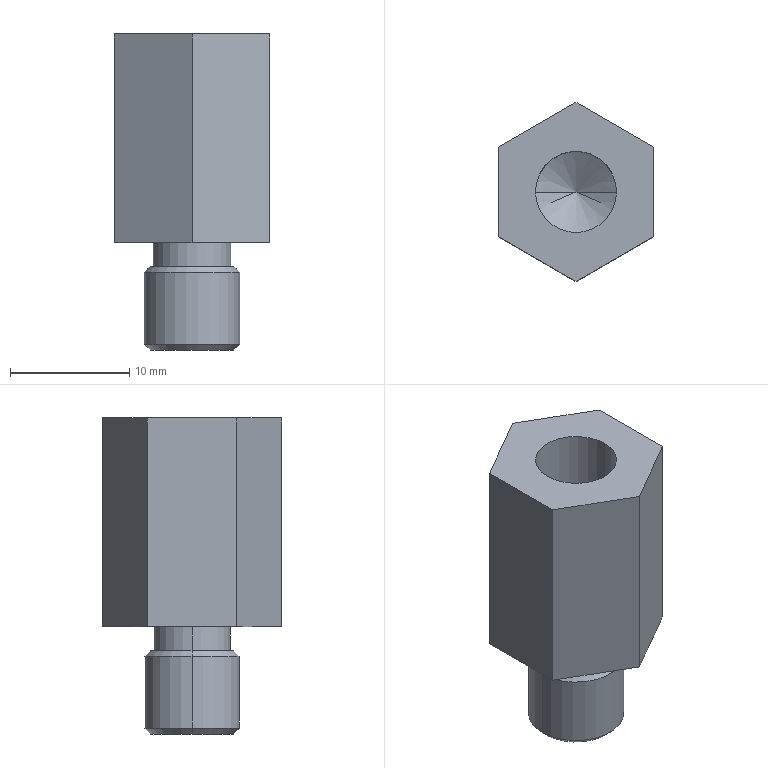Part | STEP file | M8X20 nut | 1 solid | 22 faces | box 13 x 15.011 x 26.5 mm | volume 2477 mm3 | plane 10 | cone 6 | cylinder 6 | commonest cylinder face diameters 6.5 x2 6.8 x2 8 x2
STEP:
#1=CARTESIAN_POINT('',(0.,0.,0.));
#2=DIRECTION('',(0.,0.,1.));
#3=DIRECTION('',(1.,0.,0.));
#4=AXIS2_PLACEMENT_3D('',#1,#2,#3);
#5=CARTESIAN_POINT('',(-3.5,0.,-17.75));
#6=VERTEX_POINT('',#5);
#7=CARTESIAN_POINT('',(3.5,0.,-17.75));
#8=VERTEX_POINT('',#7);
#9=CARTESIAN_POINT('',(0.,0.,-17.75));
#10=DIRECTION('',(0.,0.,-1.));
#11=DIRECTION('',(-1.,0.,0.));
#12=AXIS2_PLACEMENT_3D('',#9,#10,#11);
#13=CIRCLE('',#12,3.5);
#14=CARTESIAN_POINT('',(0.,0.,-17.75));
#15=DIRECTION('',(0.,0.,1.));
#16=DIRECTION('',(1.,0.,0.));
#17=AXIS2_PLACEMENT_3D('',#14,#15,#16);
#18=CONICAL_SURFACE('',#17,3.5,0.7854);
#19=CARTESIAN_POINT('',(3.142,0.));
#20=DIRECTION('',(-1.,0.));
#21=VECTOR('',#20,1.);
#22=LINE('',#19,#21);
#23=(GEOMETRIC_REPRESENTATION_CONTEXT(2)PARAMETRIC_REPRESENTATION_CONTEXT()REPRESENTATION_CONTEXT('',''));
#24=DEFINITIONAL_REPRESENTATION('',(#22),#23);
#25=PCURVE('',#18,#24);
#26=CARTESIAN_POINT('',(0.,0.,-17.75));
#27=DIRECTION('',(0.,0.,-1.));
#28=DIRECTION('',(-1.,0.,0.));
#29=AXIS2_PLACEMENT_3D('',#26,#27,#28);
#30=PLANE('',#29);
#31=CARTESIAN_POINT('',(0.,0.));
#32=DIRECTION('',(1.,0.));
#33=AXIS2_PLACEMENT_2D('',#31,#32);
#34=CIRCLE('',#33,3.5);
#35=(GEOMETRIC_REPRESENTATION_CONTEXT(2)PARAMETRIC_REPRESENTATION_CONTEXT()REPRESENTATION_CONTEXT('',''));
#36=DEFINITIONAL_REPRESENTATION('',(#34),#35);
#37=PCURVE('',#30,#36);
#38=SURFACE_CURVE('',#13,(#25,#37),.PCURVE_S1.);
#39=EDGE_CURVE('',#6,#8,#38,.T.);
#40=ORIENTED_EDGE('',*,*,#39,.F.);
#41=CARTESIAN_POINT('',(-4.,0.,-17.25));
#42=VERTEX_POINT('',#41);
#43=CARTESIAN_POINT('',(-3.5,0.,-17.75));
#44=DIRECTION('',(-0.7071,0.,0.7071));
#45=VECTOR('',#44,1.);
#46=LINE('',#43,#45);
#47=CARTESIAN_POINT('',(3.142,0.));
#48=DIRECTION('',(0.,1.));
#49=VECTOR('',#48,1.);
#50=LINE('',#47,#49);
#51=(GEOMETRIC_REPRESENTATION_CONTEXT(2)PARAMETRIC_REPRESENTATION_CONTEXT()REPRESENTATION_CONTEXT('',''));
#52=DEFINITIONAL_REPRESENTATION('',(#50),#51);
#53=PCURVE('',#18,#52);
#54=CARTESIAN_POINT('',(0.,0.,-17.75));
#55=DIRECTION('',(0.,0.,1.));
#56=DIRECTION('',(1.,0.,0.));
#57=AXIS2_PLACEMENT_3D('',#54,#55,#56);
#58=CONICAL_SURFACE('',#57,3.5,0.7854);
#59=CARTESIAN_POINT('',(3.142,0.));
#60=DIRECTION('',(0.,1.));
#61=VECTOR('',#60,1.);
#62=LINE('',#59,#61);
#63=(GEOMETRIC_REPRESENTATION_CONTEXT(2)PARAMETRIC_REPRESENTATION_CONTEXT()REPRESENTATION_CONTEXT('',''));
#64=DEFINITIONAL_REPRESENTATION('',(#62),#63);
#65=PCURVE('',#58,#64);
#66=SURFACE_CURVE('',#46,(#53,#65),.PCURVE_S1.);
#67=EDGE_CURVE('',#6,#42,#66,.T.);
#68=ORIENTED_EDGE('',*,*,#67,.T.);
#69=CARTESIAN_POINT('',(4.,0.,-17.25));
#70=VERTEX_POINT('',#69);
#71=CARTESIAN_POINT('',(0.,0.,-17.25));
#72=DIRECTION('',(0.,0.,1.));
#73=DIRECTION('',(-1.,0.,0.));
#74=AXIS2_PLACEMENT_3D('',#71,#72,#73);
#75=CIRCLE('',#74,4.);
#76=CARTESIAN_POINT('',(-3.142,0.5));
#77=DIRECTION('',(1.,0.));
#78=VECTOR('',#77,1.);
#79=LINE('',#76,#78);
#80=(GEOMETRIC_REPRESENTATION_CONTEXT(2)PARAMETRIC_REPRESENTATION_CONTEXT()REPRESENTATION_CONTEXT('',''));
#81=DEFINITIONAL_REPRESENTATION('',(#79),#80);
#82=PCURVE('',#18,#81);
#83=CARTESIAN_POINT('',(0.,0.,-17.75));
#84=DIRECTION('',(0.,0.,1.));
#85=DIRECTION('',(1.,0.,0.));
#86=AXIS2_PLACEMENT_3D('',#83,#84,#85);
#87=CYLINDRICAL_SURFACE('',#86,4.);
#88=CARTESIAN_POINT('',(-3.142,0.5));
#89=DIRECTION('',(1.,0.));
#90=VECTOR('',#89,1.);
#91=LINE('',#88,#90);
#92=(GEOMETRIC_REPRESENTATION_CONTEXT(2)PARAMETRIC_REPRESENTATION_CONTEXT()REPRESENTATION_CONTEXT('',''));
#93=DEFINITIONAL_REPRESENTATION('',(#91),#92);
#94=PCURVE('',#87,#93);
#95=SURFACE_CURVE('',#75,(#82,#94),.PCURVE_S1.);
#96=EDGE_CURVE('',#70,#42,#95,.T.);
#97=ORIENTED_EDGE('',*,*,#96,.F.);
#98=CARTESIAN_POINT('',(3.5,0.,-17.75));
#99=DIRECTION('',(0.7071,0.,0.7071));
#100=VECTOR('',#99,1.);
#101=LINE('',#98,#100);
#102=CARTESIAN_POINT('',(0.,0.));
#103=DIRECTION('',(0.,1.));
#104=VECTOR('',#103,1.);
#105=LINE('',#102,#104);
#106=(GEOMETRIC_REPRESENTATION_CONTEXT(2)PARAMETRIC_REPRESENTATION_CONTEXT()REPRESENTATION_CONTEXT('',''));
#107=DEFINITIONAL_REPRESENTATION('',(#105),#106);
#108=PCURVE('',#18,#107);
#109=CARTESIAN_POINT('',(6.283,0.));
#110=DIRECTION('',(0.,1.));
#111=VECTOR('',#110,1.);
#112=LINE('',#109,#111);
#113=(GEOMETRIC_REPRESENTATION_CONTEXT(2)PARAMETRIC_REPRESENTATION_CONTEXT()REPRESENTATION_CONTEXT('',''));
#114=DEFINITIONAL_REPRESENTATION('',(#112),#113);
#115=PCURVE('',#58,#114);
#116=SURFACE_CURVE('',#101,(#108,#115),.PCURVE_S1.);
#117=EDGE_CURVE('',#8,#70,#116,.T.);
#118=ORIENTED_EDGE('',*,*,#117,.F.);
#119=EDGE_LOOP('',(#40,#68,#97,#118));
#120=FACE_BOUND('',#119,.T.);
#121=ADVANCED_FACE('',(#120),#18,.T.);
#122=CARTESIAN_POINT('',(3.5,0.,-10.75));
#123=VERTEX_POINT('',#122);
#124=CARTESIAN_POINT('',(-3.5,0.,-10.75));
#125=VERTEX_POINT('',#124);
#126=CARTESIAN_POINT('',(0.,0.,-10.75));
#127=DIRECTION('',(0.,0.,1.));
#128=DIRECTION('',(-1.,0.,0.));
#129=AXIS2_PLACEMENT_3D('',#126,#127,#128);
#130=CIRCLE('',#129,3.5);
#131=CARTESIAN_POINT('',(0.,0.,-11.25));
#132=DIRECTION('',(0.,0.,-1.));
#133=DIRECTION('',(-1.,0.,0.));
#134=AXIS2_PLACEMENT_3D('',#131,#132,#133);
#135=CONICAL_SURFACE('',#134,4.,0.7854);
#136=CARTESIAN_POINT('',(6.283,-0.5));
#137=DIRECTION('',(-1.,0.));
#138=VECTOR('',#137,1.);
#139=LINE('',#136,#138);
#140=(GEOMETRIC_REPRESENTATION_CONTEXT(2)PARAMETRIC_REPRESENTATION_CONTEXT()REPRESENTATION_CONTEXT('',''));
#141=DEFINITIONAL_REPRESENTATION('',(#139),#140);
#142=PCURVE('',#135,#141);
#143=CARTESIAN_POINT('',(0.,0.,-10.75));
#144=DIRECTION('',(0.,0.,-1.));
#145=DIRECTION('',(-1.,0.,0.));
#146=AXIS2_PLACEMENT_3D('',#143,#144,#145);
#147=PLANE('',#146);
#148=CARTESIAN_POINT('',(3.5,0.));
#149=CARTESIAN_POINT('',(3.5,-6.062));
#150=CARTESIAN_POINT('',(-1.75,-3.031));
#151=CARTESIAN_POINT('',(-7.,0.));
#152=CARTESIAN_POINT('',(-1.75,3.031));
#153=CARTESIAN_POINT('',(3.5,6.062));
#154=CARTESIAN_POINT('',(3.5,0.));
#155=(BOUNDED_CURVE()B_SPLINE_CURVE(2,(#148,#149,#150,#151,#152,#153,#154),.UNSPECIFIED.,.T.,.F.)B_SPLINE_CURVE_WITH_KNOTS((1,2,2,2,2,1),(-2.094,0.,2.094,4.189,6.283,8.378),.UNSPECIFIED.)CURVE()GEOMETRIC_REPRESENTATION_ITEM()RATIONAL_B_SPLINE_CURVE((1.,0.5,1.,0.5,1.,0.5,1.))REPRESENTATION_ITEM(''));
#156=(GEOMETRIC_REPRESENTATION_CONTEXT(2)PARAMETRIC_REPRESENTATION_CONTEXT()REPRESENTATION_CONTEXT('',''));
#157=DEFINITIONAL_REPRESENTATION('',(#155),#156);
#158=PCURVE('',#147,#157);
#159=SURFACE_CURVE('',#130,(#142,#158),.PCURVE_S1.);
#160=EDGE_CURVE('',#123,#125,#159,.T.);
#161=ORIENTED_EDGE('',*,*,#160,.F.);
#162=CARTESIAN_POINT('',(4.,0.,-11.25));
#163=VERTEX_POINT('',#162);
#164=CARTESIAN_POINT('',(4.,0.,-11.25));
#165=DIRECTION('',(0.7071,0.,-0.7071));
#166=VECTOR('',#165,1.);
#167=LINE('',#164,#166);
#168=CARTESIAN_POINT('',(3.142,0.));
#169=DIRECTION('',(0.,1.));
#170=VECTOR('',#169,1.);
#171=LINE('',#168,#170);
#172=(GEOMETRIC_REPRESENTATION_CONTEXT(2)PARAMETRIC_REPRESENTATION_CONTEXT()REPRESENTATION_CONTEXT('',''));
#173=DEFINITIONAL_REPRESENTATION('',(#171),#172);
#174=PCURVE('',#135,#173);
#175=CARTESIAN_POINT('',(0.,0.,-11.25));
#176=DIRECTION('',(0.,0.,-1.));
#177=DIRECTION('',(-1.,0.,0.));
#178=AXIS2_PLACEMENT_3D('',#175,#176,#177);
#179=CONICAL_SURFACE('',#178,4.,0.7854);
#180=CARTESIAN_POINT('',(3.142,0.));
#181=DIRECTION('',(0.,1.));
#182=VECTOR('',#181,1.);
#183=LINE('',#180,#182);
#184=(GEOMETRIC_REPRESENTATION_CONTEXT(2)PARAMETRIC_REPRESENTATION_CONTEXT()REPRESENTATION_CONTEXT('',''));
#185=DEFINITIONAL_REPRESENTATION('',(#183),#184);
#186=PCURVE('',#179,#185);
#187=SURFACE_CURVE('',#167,(#174,#186),.PCURVE_S1.);
#188=EDGE_CURVE('',#123,#163,#187,.T.);
#189=ORIENTED_EDGE('',*,*,#188,.T.);
#190=CARTESIAN_POINT('',(-4.,0.,-11.25));
#191=VERTEX_POINT('',#190);
#192=CARTESIAN_POINT('',(0.,0.,-11.25));
#193=DIRECTION('',(0.,0.,-1.));
#194=DIRECTION('',(-1.,0.,0.));
#195=AXIS2_PLACEMENT_3D('',#192,#193,#194);
#196=CIRCLE('',#195,4.);
#197=CARTESIAN_POINT('',(0.,0.));
#198=DIRECTION('',(1.,0.));
#199=VECTOR('',#198,1.);
#200=LINE('',#197,#199);
#201=(GEOMETRIC_REPRESENTATION_CONTEXT(2)PARAMETRIC_REPRESENTATION_CONTEXT()REPRESENTATION_CONTEXT('',''));
#202=DEFINITIONAL_REPRESENTATION('',(#200),#201);
#203=PCURVE('',#135,#202);
#204=CARTESIAN_POINT('',(3.142,6.5));
#205=DIRECTION('',(-1.,0.));
#206=VECTOR('',#205,1.);
#207=LINE('',#204,#206);
#208=(GEOMETRIC_REPRESENTATION_CONTEXT(2)PARAMETRIC_REPRESENTATION_CONTEXT()REPRESENTATION_CONTEXT('',''));
#209=DEFINITIONAL_REPRESENTATION('',(#207),#208);
#210=PCURVE('',#87,#209);
#211=SURFACE_CURVE('',#196,(#203,#210),.PCURVE_S1.);
#212=EDGE_CURVE('',#191,#163,#211,.T.);
#213=ORIENTED_EDGE('',*,*,#212,.F.);
#214=CARTESIAN_POINT('',(-4.,0.,-11.25));
#215=DIRECTION('',(-0.7071,0.,-0.7071));
#216=VECTOR('',#215,1.);
#217=LINE('',#214,#216);
#218=CARTESIAN_POINT('',(0.,0.));
#219=DIRECTION('',(0.,1.));
#220=VECTOR('',#219,1.);
#221=LINE('',#218,#220);
#222=(GEOMETRIC_REPRESENTATION_CONTEXT(2)PARAMETRIC_REPRESENTATION_CONTEXT()REPRESENTATION_CONTEXT('',''));
#223=DEFINITIONAL_REPRESENTATION('',(#221),#222);
#224=PCURVE('',#135,#223);
#225=CARTESIAN_POINT('',(6.283,0.));
#226=DIRECTION('',(0.,1.));
#227=VECTOR('',#226,1.);
#228=LINE('',#225,#227);
#229=(GEOMETRIC_REPRESENTATION_CONTEXT(2)PARAMETRIC_REPRESENTATION_CONTEXT()REPRESENTATION_CONTEXT('',''));
#230=DEFINITIONAL_REPRESENTATION('',(#228),#229);
#231=PCURVE('',#179,#230);
#232=SURFACE_CURVE('',#217,(#224,#231),.PCURVE_S1.);
#233=EDGE_CURVE('',#125,#191,#232,.T.);
#234=ORIENTED_EDGE('',*,*,#233,.F.);
#235=EDGE_LOOP('',(#161,#189,#213,#234));
#236=FACE_BOUND('',#235,.T.);
#237=ADVANCED_FACE('',(#236),#135,.T.);
#238=ORIENTED_EDGE('',*,*,#96,.T.);
#239=CARTESIAN_POINT('',(-4.,0.,-17.75));
#240=DIRECTION('',(0.,0.,1.));
#241=VECTOR('',#240,1.);
#242=LINE('',#239,#241);
#243=CARTESIAN_POINT('',(3.142,0.));
#244=DIRECTION('',(0.,1.));
#245=VECTOR('',#244,1.);
#246=LINE('',#243,#245);
#247=(GEOMETRIC_REPRESENTATION_CONTEXT(2)PARAMETRIC_REPRESENTATION_CONTEXT()REPRESENTATION_CONTEXT('',''));
#248=DEFINITIONAL_REPRESENTATION('',(#246),#247);
#249=PCURVE('',#87,#248);
#250=CARTESIAN_POINT('',(0.,0.,-17.75));
#251=DIRECTION('',(0.,0.,1.));
#252=DIRECTION('',(1.,0.,0.));
#253=AXIS2_PLACEMENT_3D('',#250,#251,#252);
#254=CYLINDRICAL_SURFACE('',#253,4.);
#255=CARTESIAN_POINT('',(3.142,0.));
#256=DIRECTION('',(0.,1.));
#257=VECTOR('',#256,1.);
#258=LINE('',#255,#257);
#259=(GEOMETRIC_REPRESENTATION_CONTEXT(2)PARAMETRIC_REPRESENTATION_CONTEXT()REPRESENTATION_CONTEXT('',''));
#260=DEFINITIONAL_REPRESENTATION('',(#258),#259);
#261=PCURVE('',#254,#260);
#262=SURFACE_CURVE('',#242,(#249,#261),.PCURVE_S1.);
#263=EDGE_CURVE('',#42,#191,#262,.T.);
#264=ORIENTED_EDGE('',*,*,#263,.T.);
#265=ORIENTED_EDGE('',*,*,#212,.T.);
#266=CARTESIAN_POINT('',(4.,0.,-17.75));
#267=DIRECTION('',(0.,0.,1.));
#268=VECTOR('',#267,1.);
#269=LINE('',#266,#268);
#270=CARTESIAN_POINT('',(0.,0.));
#271=DIRECTION('',(0.,1.));
#272=VECTOR('',#271,1.);
#273=LINE('',#270,#272);
#274=(GEOMETRIC_REPRESENTATION_CONTEXT(2)PARAMETRIC_REPRESENTATION_CONTEXT()REPRESENTATION_CONTEXT('',''));
#275=DEFINITIONAL_REPRESENTATION('',(#273),#274);
#276=PCURVE('',#87,#275);
#277=CARTESIAN_POINT('',(6.283,0.));
#278=DIRECTION('',(0.,1.));
#279=VECTOR('',#278,1.);
#280=LINE('',#277,#279);
#281=(GEOMETRIC_REPRESENTATION_CONTEXT(2)PARAMETRIC_REPRESENTATION_CONTEXT()REPRESENTATION_CONTEXT('',''));
#282=DEFINITIONAL_REPRESENTATION('',(#280),#281);
#283=PCURVE('',#254,#282);
#284=SURFACE_CURVE('',#269,(#276,#283),.PCURVE_S1.);
#285=EDGE_CURVE('',#70,#163,#284,.T.);
#286=ORIENTED_EDGE('',*,*,#285,.F.);
#287=EDGE_LOOP('',(#238,#264,#265,#286));
#288=FACE_BOUND('',#287,.T.);
#289=ADVANCED_FACE('',(#288),#87,.T.);
#290=CARTESIAN_POINT('',(-3.25,0.,-10.75));
#291=VERTEX_POINT('',#290);
#292=CARTESIAN_POINT('',(3.25,0.,-10.75));
#293=VERTEX_POINT('',#292);
#294=CARTESIAN_POINT('',(0.,0.,-10.75));
#295=DIRECTION('',(0.,0.,-1.));
#296=DIRECTION('',(-1.,0.,0.));
#297=AXIS2_PLACEMENT_3D('',#294,#295,#296);
#298=CIRCLE('',#297,3.25);
#299=CARTESIAN_POINT('',(0.,0.,-10.75));
#300=DIRECTION('',(0.,0.,1.));
#301=DIRECTION('',(1.,0.,0.));
#302=AXIS2_PLACEMENT_3D('',#299,#300,#301);
#303=CYLINDRICAL_SURFACE('',#302,3.25);
#304=CARTESIAN_POINT('',(3.142,0.));
#305=DIRECTION('',(-1.,0.));
#306=VECTOR('',#305,1.);
#307=LINE('',#304,#306);
#308=(GEOMETRIC_REPRESENTATION_CONTEXT(2)PARAMETRIC_REPRESENTATION_CONTEXT()REPRESENTATION_CONTEXT('',''));
#309=DEFINITIONAL_REPRESENTATION('',(#307),#308);
#310=PCURVE('',#303,#309);
#311=CARTESIAN_POINT('',(0.,0.));
#312=DIRECTION('',(1.,0.));
#313=AXIS2_PLACEMENT_2D('',#311,#312);
#314=CIRCLE('',#313,3.25);
#315=(GEOMETRIC_REPRESENTATION_CONTEXT(2)PARAMETRIC_REPRESENTATION_CONTEXT()REPRESENTATION_CONTEXT('',''));
#316=DEFINITIONAL_REPRESENTATION('',(#314),#315);
#317=PCURVE('',#147,#316);
#318=SURFACE_CURVE('',#298,(#310,#317),.PCURVE_S1.);
#319=EDGE_CURVE('',#291,#293,#318,.T.);
#320=ORIENTED_EDGE('',*,*,#319,.F.);
#321=CARTESIAN_POINT('',(-3.25,0.,-8.75));
#322=VERTEX_POINT('',#321);
#323=CARTESIAN_POINT('',(-3.25,0.,-10.75));
#324=DIRECTION('',(0.,0.,1.));
#325=VECTOR('',#324,1.);
#326=LINE('',#323,#325);
#327=CARTESIAN_POINT('',(3.142,0.));
#328=DIRECTION('',(0.,1.));
#329=VECTOR('',#328,1.);
#330=LINE('',#327,#329);
#331=(GEOMETRIC_REPRESENTATION_CONTEXT(2)PARAMETRIC_REPRESENTATION_CONTEXT()REPRESENTATION_CONTEXT('',''));
#332=DEFINITIONAL_REPRESENTATION('',(#330),#331);
#333=PCURVE('',#303,#332);
#334=CARTESIAN_POINT('',(0.,0.,-10.75));
#335=DIRECTION('',(0.,0.,1.));
#336=DIRECTION('',(1.,0.,0.));
#337=AXIS2_PLACEMENT_3D('',#334,#335,#336);
#338=CYLINDRICAL_SURFACE('',#337,3.25);
#339=CARTESIAN_POINT('',(3.142,0.));
#340=DIRECTION('',(0.,1.));
#341=VECTOR('',#340,1.);
#342=LINE('',#339,#341);
#343=(GEOMETRIC_REPRESENTATION_CONTEXT(2)PARAMETRIC_REPRESENTATION_CONTEXT()REPRESENTATION_CONTEXT('',''));
#344=DEFINITIONAL_REPRESENTATION('',(#342),#343);
#345=PCURVE('',#338,#344);
#346=SURFACE_CURVE('',#326,(#333,#345),.PCURVE_S1.);
#347=EDGE_CURVE('',#291,#322,#346,.T.);
#348=ORIENTED_EDGE('',*,*,#347,.T.);
#349=CARTESIAN_POINT('',(3.25,0.,-8.75));
#350=VERTEX_POINT('',#349);
#351=CARTESIAN_POINT('',(0.,0.,-8.75));
#352=DIRECTION('',(0.,0.,-1.));
#353=DIRECTION('',(1.,0.,0.));
#354=AXIS2_PLACEMENT_3D('',#351,#352,#353);
#355=CIRCLE('',#354,3.25);
#356=CARTESIAN_POINT('',(6.283,2.));
#357=DIRECTION('',(-1.,0.));
#358=VECTOR('',#357,1.);
#359=LINE('',#356,#358);
#360=(GEOMETRIC_REPRESENTATION_CONTEXT(2)PARAMETRIC_REPRESENTATION_CONTEXT()REPRESENTATION_CONTEXT('',''));
#361=DEFINITIONAL_REPRESENTATION('',(#359),#360);
#362=PCURVE('',#303,#361);
#363=CARTESIAN_POINT('',(0.,0.,-8.75));
#364=DIRECTION('',(0.,0.,1.));
#365=DIRECTION('',(1.,0.,0.));
#366=AXIS2_PLACEMENT_3D('',#363,#364,#365);
#367=PLANE('',#366);
#368=CARTESIAN_POINT('',(3.25,0.));
#369=CARTESIAN_POINT('',(3.25,-5.629));
#370=CARTESIAN_POINT('',(-1.625,-2.815));
#371=CARTESIAN_POINT('',(-6.5,0.));
#372=CARTESIAN_POINT('',(-1.625,2.815));
#373=CARTESIAN_POINT('',(3.25,5.629));
#374=CARTESIAN_POINT('',(3.25,0.));
#375=(BOUNDED_CURVE()B_SPLINE_CURVE(2,(#368,#369,#370,#371,#372,#373,#374),.UNSPECIFIED.,.T.,.F.)B_SPLINE_CURVE_WITH_KNOTS((1,2,2,2,2,1),(-2.094,0.,2.094,4.189,6.283,8.378),.UNSPECIFIED.)CURVE()GEOMETRIC_REPRESENTATION_ITEM()RATIONAL_B_SPLINE_CURVE((1.,0.5,1.,0.5,1.,0.5,1.))REPRESENTATION_ITEM(''));
#376=(GEOMETRIC_REPRESENTATION_CONTEXT(2)PARAMETRIC_REPRESENTATION_CONTEXT()REPRESENTATION_CONTEXT('',''));
#377=DEFINITIONAL_REPRESENTATION('',(#375),#376);
#378=PCURVE('',#367,#377);
#379=SURFACE_CURVE('',#355,(#362,#378),.PCURVE_S1.);
#380=EDGE_CURVE('',#322,#350,#379,.T.);
#381=ORIENTED_EDGE('',*,*,#380,.T.);
#382=CARTESIAN_POINT('',(3.25,0.,-10.75));
#383=DIRECTION('',(0.,0.,1.));
#384=VECTOR('',#383,1.);
#385=LINE('',#382,#384);
#386=CARTESIAN_POINT('',(0.,0.));
#387=DIRECTION('',(0.,1.));
#388=VECTOR('',#387,1.);
#389=LINE('',#386,#388);
#390=(GEOMETRIC_REPRESENTATION_CONTEXT(2)PARAMETRIC_REPRESENTATION_CONTEXT()REPRESENTATION_CONTEXT('',''));
#391=DEFINITIONAL_REPRESENTATION('',(#389),#390);
#392=PCURVE('',#303,#391);
#393=CARTESIAN_POINT('',(6.283,0.));
#394=DIRECTION('',(0.,1.));
#395=VECTOR('',#394,1.);
#396=LINE('',#393,#395);
#397=(GEOMETRIC_REPRESENTATION_CONTEXT(2)PARAMETRIC_REPRESENTATION_CONTEXT()REPRESENTATION_CONTEXT('',''));
#398=DEFINITIONAL_REPRESENTATION('',(#396),#397);
#399=PCURVE('',#338,#398);
#400=SURFACE_CURVE('',#385,(#392,#399),.PCURVE_S1.);
#401=EDGE_CURVE('',#293,#350,#400,.T.);
#402=ORIENTED_EDGE('',*,*,#401,.F.);
#403=EDGE_LOOP('',(#320,#348,#381,#402));
#404=FACE_BOUND('',#403,.T.);
#405=ADVANCED_FACE('',(#404),#303,.T.);
#406=CARTESIAN_POINT('',(3.4,0.,-4.25));
#407=VERTEX_POINT('',#406);
#408=CARTESIAN_POINT('',(3.4,0.,8.75));
#409=VERTEX_POINT('',#408);
#410=CARTESIAN_POINT('',(3.4,0.,8.75));
#411=DIRECTION('',(0.,0.,1.));
#412=VECTOR('',#411,1.);
#413=LINE('',#410,#412);
#414=CARTESIAN_POINT('',(0.,0.,8.75));
#415=DIRECTION('',(0.,0.,1.));
#416=DIRECTION('',(1.,0.,0.));
#417=AXIS2_PLACEMENT_3D('',#414,#415,#416);
#418=CYLINDRICAL_SURFACE('',#417,3.4);
#419=CARTESIAN_POINT('',(6.283,0.));
#420=DIRECTION('',(0.,1.));
#421=VECTOR('',#420,1.);
#422=LINE('',#419,#421);
#423=(GEOMETRIC_REPRESENTATION_CONTEXT(2)PARAMETRIC_REPRESENTATION_CONTEXT()REPRESENTATION_CONTEXT('',''));
#424=DEFINITIONAL_REPRESENTATION('',(#422),#423);
#425=PCURVE('',#418,#424);
#426=CARTESIAN_POINT('',(0.,0.,8.75));
#427=DIRECTION('',(0.,0.,1.));
#428=DIRECTION('',(1.,0.,0.));
#429=AXIS2_PLACEMENT_3D('',#426,#427,#428);
#430=CYLINDRICAL_SURFACE('',#429,3.4);
#431=CARTESIAN_POINT('',(0.,0.));
#432=DIRECTION('',(0.,1.));
#433=VECTOR('',#432,1.);
#434=LINE('',#431,#433);
#435=(GEOMETRIC_REPRESENTATION_CONTEXT(2)PARAMETRIC_REPRESENTATION_CONTEXT()REPRESENTATION_CONTEXT('',''));
#436=DEFINITIONAL_REPRESENTATION('',(#434),#435);
#437=PCURVE('',#430,#436);
#438=SURFACE_CURVE('',#413,(#425,#437),.PCURVE_S1.);
#439=EDGE_CURVE('',#407,#409,#438,.T.);
#440=ORIENTED_EDGE('',*,*,#439,.T.);
#441=CARTESIAN_POINT('',(-3.4,0.,8.75));
#442=VERTEX_POINT('',#441);
#443=CARTESIAN_POINT('',(0.,0.,8.75));
#444=DIRECTION('',(0.,0.,1.));
#445=DIRECTION('',(1.,0.,0.));
#446=AXIS2_PLACEMENT_3D('',#443,#444,#445);
#447=CIRCLE('',#446,3.4);
#448=CARTESIAN_POINT('',(0.,0.));
#449=DIRECTION('',(1.,0.));
#450=VECTOR('',#449,1.);
#451=LINE('',#448,#450);
#452=(GEOMETRIC_REPRESENTATION_CONTEXT(2)PARAMETRIC_REPRESENTATION_CONTEXT()REPRESENTATION_CONTEXT('',''));
#453=DEFINITIONAL_REPRESENTATION('',(#451),#452);
#454=PCURVE('',#418,#453);
#455=CARTESIAN_POINT('',(0.,0.,8.75));
#456=DIRECTION('',(0.,0.,1.));
#457=DIRECTION('',(1.,0.,0.));
#458=AXIS2_PLACEMENT_3D('',#455,#456,#457);
#459=PLANE('',#458);
#460=CARTESIAN_POINT('',(0.,0.));
#461=DIRECTION('',(1.,0.));
#462=AXIS2_PLACEMENT_2D('',#460,#461);
#463=CIRCLE('',#462,3.4);
#464=(GEOMETRIC_REPRESENTATION_CONTEXT(2)PARAMETRIC_REPRESENTATION_CONTEXT()REPRESENTATION_CONTEXT('',''));
#465=DEFINITIONAL_REPRESENTATION('',(#463),#464);
#466=PCURVE('',#459,#465);
#467=SURFACE_CURVE('',#447,(#454,#466),.PCURVE_S1.);
#468=EDGE_CURVE('',#442,#409,#467,.T.);
#469=ORIENTED_EDGE('',*,*,#468,.F.);
#470=CARTESIAN_POINT('',(-3.4,0.,-4.25));
#471=VERTEX_POINT('',#470);
#472=CARTESIAN_POINT('',(-3.4,0.,8.75));
#473=DIRECTION('',(0.,0.,1.));
#474=VECTOR('',#473,1.);
#475=LINE('',#472,#474);
#476=CARTESIAN_POINT('',(3.142,0.));
#477=DIRECTION('',(0.,1.));
#478=VECTOR('',#477,1.);
#479=LINE('',#476,#478);
#480=(GEOMETRIC_REPRESENTATION_CONTEXT(2)PARAMETRIC_REPRESENTATION_CONTEXT()REPRESENTATION_CONTEXT('',''));
#481=DEFINITIONAL_REPRESENTATION('',(#479),#480);
#482=PCURVE('',#418,#481);
#483=CARTESIAN_POINT('',(3.142,0.));
#484=DIRECTION('',(0.,1.));
#485=VECTOR('',#484,1.);
#486=LINE('',#483,#485);
#487=(GEOMETRIC_REPRESENTATION_CONTEXT(2)PARAMETRIC_REPRESENTATION_CONTEXT()REPRESENTATION_CONTEXT('',''));
#488=DEFINITIONAL_REPRESENTATION('',(#486),#487);
#489=PCURVE('',#430,#488);
#490=SURFACE_CURVE('',#475,(#482,#489),.PCURVE_S1.);
#491=EDGE_CURVE('',#471,#442,#490,.T.);
#492=ORIENTED_EDGE('',*,*,#491,.F.);
#493=CARTESIAN_POINT('',(0.,0.,-4.25));
#494=DIRECTION('',(0.,0.,1.));
#495=DIRECTION('',(1.,0.,0.));
#496=AXIS2_PLACEMENT_3D('',#493,#494,#495);
#497=CIRCLE('',#496,3.4);
#498=CARTESIAN_POINT('',(0.,-13.));
#499=DIRECTION('',(1.,0.));
#500=VECTOR('',#499,1.);
#501=LINE('',#498,#500);
#502=(GEOMETRIC_REPRESENTATION_CONTEXT(2)PARAMETRIC_REPRESENTATION_CONTEXT()REPRESENTATION_CONTEXT('',''));
#503=DEFINITIONAL_REPRESENTATION('',(#501),#502);
#504=PCURVE('',#418,#503);
#505=CARTESIAN_POINT('',(0.,0.,-4.25));
#506=DIRECTION('',(0.,0.,1.));
#507=DIRECTION('',(1.,0.,0.));
#508=AXIS2_PLACEMENT_3D('',#505,#506,#507);
#509=CONICAL_SURFACE('',#508,3.4,1.03);
#510=CARTESIAN_POINT('',(0.,0.));
#511=DIRECTION('',(1.,0.));
#512=VECTOR('',#511,1.);
#513=LINE('',#510,#512);
#514=(GEOMETRIC_REPRESENTATION_CONTEXT(2)PARAMETRIC_REPRESENTATION_CONTEXT()REPRESENTATION_CONTEXT('',''));
#515=DEFINITIONAL_REPRESENTATION('',(#513),#514);
#516=PCURVE('',#509,#515);
#517=SURFACE_CURVE('',#497,(#504,#516),.PCURVE_S1.);
#518=EDGE_CURVE('',#471,#407,#517,.T.);
#519=ORIENTED_EDGE('',*,*,#518,.T.);
#520=EDGE_LOOP('',(#440,#469,#492,#519));
#521=FACE_BOUND('',#520,.F.);
#522=ADVANCED_FACE('',(#521),#418,.F.);
#523=ORIENTED_EDGE('',*,*,#518,.F.);
#524=CARTESIAN_POINT('',(0.,0.,-6.293));
#525=VERTEX_POINT('',#524);
#526=CARTESIAN_POINT('',(-3.4,0.,-4.25));
#527=DIRECTION('',(-0.8572,0.,0.515));
#528=VECTOR('',#527,1.);
#529=LINE('',#526,#528);
#530=CARTESIAN_POINT('',(3.142,0.));
#531=DIRECTION('',(0.,1.));
#532=VECTOR('',#531,1.);
#533=LINE('',#530,#532);
#534=(GEOMETRIC_REPRESENTATION_CONTEXT(2)PARAMETRIC_REPRESENTATION_CONTEXT()REPRESENTATION_CONTEXT('',''));
#535=DEFINITIONAL_REPRESENTATION('',(#533),#534);
#536=PCURVE('',#509,#535);
#537=CARTESIAN_POINT('',(0.,0.,-4.25));
#538=DIRECTION('',(0.,0.,1.));
#539=DIRECTION('',(1.,0.,0.));
#540=AXIS2_PLACEMENT_3D('',#537,#538,#539);
#541=CONICAL_SURFACE('',#540,3.4,1.03);
#542=CARTESIAN_POINT('',(3.142,0.));
#543=DIRECTION('',(0.,1.));
#544=VECTOR('',#543,1.);
#545=LINE('',#542,#544);
#546=(GEOMETRIC_REPRESENTATION_CONTEXT(2)PARAMETRIC_REPRESENTATION_CONTEXT()REPRESENTATION_CONTEXT('',''));
#547=DEFINITIONAL_REPRESENTATION('',(#545),#546);
#548=PCURVE('',#541,#547);
#549=SURFACE_CURVE('',#529,(#536,#548),.PCURVE_S1.);
#550=EDGE_CURVE('',#525,#471,#549,.T.);
#551=ORIENTED_EDGE('',*,*,#550,.F.);
#552=CARTESIAN_POINT('',(3.4,0.,-4.25));
#553=DIRECTION('',(0.8572,0.,0.515));
#554=VECTOR('',#553,1.);
#555=LINE('',#552,#554);
#556=CARTESIAN_POINT('',(6.283,0.));
#557=DIRECTION('',(0.,1.));
#558=VECTOR('',#557,1.);
#559=LINE('',#556,#558);
#560=(GEOMETRIC_REPRESENTATION_CONTEXT(2)PARAMETRIC_REPRESENTATION_CONTEXT()REPRESENTATION_CONTEXT('',''));
#561=DEFINITIONAL_REPRESENTATION('',(#559),#560);
#562=PCURVE('',#509,#561);
#563=CARTESIAN_POINT('',(0.,0.));
#564=DIRECTION('',(0.,1.));
#565=VECTOR('',#564,1.);
#566=LINE('',#563,#565);
#567=(GEOMETRIC_REPRESENTATION_CONTEXT(2)PARAMETRIC_REPRESENTATION_CONTEXT()REPRESENTATION_CONTEXT('',''));
#568=DEFINITIONAL_REPRESENTATION('',(#566),#567);
#569=PCURVE('',#541,#568);
#570=SURFACE_CURVE('',#555,(#562,#569),.PCURVE_S1.);
#571=EDGE_CURVE('',#525,#407,#570,.T.);
#572=ORIENTED_EDGE('',*,*,#571,.T.);
#573=EDGE_LOOP('',(#523,#551,#572));
#574=FACE_BOUND('',#573,.F.);
#575=ADVANCED_FACE('',(#574),#509,.F.);
#576=CARTESIAN_POINT('',(-6.5,-3.753,-8.75));
#577=VERTEX_POINT('',#576);
#578=CARTESIAN_POINT('',(0.,-7.506,-8.75));
#579=VERTEX_POINT('',#578);
#580=CARTESIAN_POINT('',(-6.5,-3.753,-8.75));
#581=DIRECTION('',(0.866,-0.5,0.));
#582=VECTOR('',#581,1.);
#583=LINE('',#580,#582);
#584=CARTESIAN_POINT('',(-6.5,-3.753));
#585=DIRECTION('',(0.866,-0.5));
#586=VECTOR('',#585,1.);
#587=LINE('',#584,#586);
#588=(GEOMETRIC_REPRESENTATION_CONTEXT(2)PARAMETRIC_REPRESENTATION_CONTEXT()REPRESENTATION_CONTEXT('',''));
#589=DEFINITIONAL_REPRESENTATION('',(#587),#588);
#590=PCURVE('',#367,#589);
#591=CARTESIAN_POINT('',(-6.5,-3.753,8.75));
#592=DIRECTION('',(0.5,0.866,0.));
#593=DIRECTION('',(-0.866,0.5,0.));
#594=AXIS2_PLACEMENT_3D('',#591,#592,#593);
#595=PLANE('',#594);
#596=CARTESIAN_POINT('',(0.,-17.5));
#597=DIRECTION('',(-1.,0.));
#598=VECTOR('',#597,1.);
#599=LINE('',#596,#598);
#600=(GEOMETRIC_REPRESENTATION_CONTEXT(2)PARAMETRIC_REPRESENTATION_CONTEXT()REPRESENTATION_CONTEXT('',''));
#601=DEFINITIONAL_REPRESENTATION('',(#599),#600);
#602=PCURVE('',#595,#601);
#603=SURFACE_CURVE('',#583,(#590,#602),.PCURVE_S1.);
#604=EDGE_CURVE('',#577,#579,#603,.T.);
#605=ORIENTED_EDGE('',*,*,#604,.F.);
#606=CARTESIAN_POINT('',(-6.5,3.753,-8.75));
#607=VERTEX_POINT('',#606);
#608=CARTESIAN_POINT('',(-6.5,3.753,-8.75));
#609=DIRECTION('',(0.,-1.,0.));
#610=VECTOR('',#609,1.);
#611=LINE('',#608,#610);
#612=CARTESIAN_POINT('',(-6.5,3.753));
#613=DIRECTION('',(0.,-1.));
#614=VECTOR('',#613,1.);
#615=LINE('',#612,#614);
#616=(GEOMETRIC_REPRESENTATION_CONTEXT(2)PARAMETRIC_REPRESENTATION_CONTEXT()REPRESENTATION_CONTEXT('',''));
#617=DEFINITIONAL_REPRESENTATION('',(#615),#616);
#618=PCURVE('',#367,#617);
#619=CARTESIAN_POINT('',(-6.5,3.753,8.75));
#620=DIRECTION('',(1.,0.,0.));
#621=DIRECTION('',(0.,1.,0.));
#622=AXIS2_PLACEMENT_3D('',#619,#620,#621);
#623=PLANE('',#622);
#624=CARTESIAN_POINT('',(0.,-17.5));
#625=DIRECTION('',(-1.,0.));
#626=VECTOR('',#625,1.);
#627=LINE('',#624,#626);
#628=(GEOMETRIC_REPRESENTATION_CONTEXT(2)PARAMETRIC_REPRESENTATION_CONTEXT()REPRESENTATION_CONTEXT('',''));
#629=DEFINITIONAL_REPRESENTATION('',(#627),#628);
#630=PCURVE('',#623,#629);
#631=SURFACE_CURVE('',#611,(#618,#630),.PCURVE_S1.);
#632=EDGE_CURVE('',#607,#577,#631,.T.);
#633=ORIENTED_EDGE('',*,*,#632,.F.);
#634=CARTESIAN_POINT('',(0.,7.506,-8.75));
#635=VERTEX_POINT('',#634);
#636=CARTESIAN_POINT('',(0.,7.506,-8.75));
#637=DIRECTION('',(-0.866,-0.5,0.));
#638=VECTOR('',#637,1.);
#639=LINE('',#636,#638);
#640=CARTESIAN_POINT('',(0.,7.506));
#641=DIRECTION('',(-0.866,-0.5));
#642=VECTOR('',#641,1.);
#643=LINE('',#640,#642);
#644=(GEOMETRIC_REPRESENTATION_CONTEXT(2)PARAMETRIC_REPRESENTATION_CONTEXT()REPRESENTATION_CONTEXT('',''));
#645=DEFINITIONAL_REPRESENTATION('',(#643),#644);
#646=PCURVE('',#367,#645);
#647=CARTESIAN_POINT('',(0.,7.506,8.75));
#648=DIRECTION('',(0.5,-0.866,0.));
#649=DIRECTION('',(0.866,0.5,0.));
#650=AXIS2_PLACEMENT_3D('',#647,#648,#649);
#651=PLANE('',#650);
#652=CARTESIAN_POINT('',(0.,-17.5));
#653=DIRECTION('',(-1.,0.));
#654=VECTOR('',#653,1.);
#655=LINE('',#652,#654);
#656=(GEOMETRIC_REPRESENTATION_CONTEXT(2)PARAMETRIC_REPRESENTATION_CONTEXT()REPRESENTATION_CONTEXT('',''));
#657=DEFINITIONAL_REPRESENTATION('',(#655),#656);
#658=PCURVE('',#651,#657);
#659=SURFACE_CURVE('',#639,(#646,#658),.PCURVE_S1.);
#660=EDGE_CURVE('',#635,#607,#659,.T.);
#661=ORIENTED_EDGE('',*,*,#660,.F.);
#662=CARTESIAN_POINT('',(6.5,3.753,-8.75));
#663=VERTEX_POINT('',#662);
#664=CARTESIAN_POINT('',(6.5,3.753,-8.75));
#665=DIRECTION('',(-0.866,0.5,0.));
#666=VECTOR('',#665,1.);
#667=LINE('',#664,#666);
#668=CARTESIAN_POINT('',(6.5,3.753));
#669=DIRECTION('',(-0.866,0.5));
#670=VECTOR('',#669,1.);
#671=LINE('',#668,#670);
#672=(GEOMETRIC_REPRESENTATION_CONTEXT(2)PARAMETRIC_REPRESENTATION_CONTEXT()REPRESENTATION_CONTEXT('',''));
#673=DEFINITIONAL_REPRESENTATION('',(#671),#672);
#674=PCURVE('',#367,#673);
#675=CARTESIAN_POINT('',(6.5,3.753,8.75));
#676=DIRECTION('',(-0.5,-0.866,0.));
#677=DIRECTION('',(0.866,-0.5,0.));
#678=AXIS2_PLACEMENT_3D('',#675,#676,#677);
#679=PLANE('',#678);
#680=CARTESIAN_POINT('',(0.,-17.5));
#681=DIRECTION('',(-1.,0.));
#682=VECTOR('',#681,1.);
#683=LINE('',#680,#682);
#684=(GEOMETRIC_REPRESENTATION_CONTEXT(2)PARAMETRIC_REPRESENTATION_CONTEXT()REPRESENTATION_CONTEXT('',''));
#685=DEFINITIONAL_REPRESENTATION('',(#683),#684);
#686=PCURVE('',#679,#685);
#687=SURFACE_CURVE('',#667,(#674,#686),.PCURVE_S1.);
#688=EDGE_CURVE('',#663,#635,#687,.T.);
#689=ORIENTED_EDGE('',*,*,#688,.F.);
#690=CARTESIAN_POINT('',(6.5,-3.753,-8.75));
#691=VERTEX_POINT('',#690);
#692=CARTESIAN_POINT('',(6.5,-3.753,-8.75));
#693=DIRECTION('',(0.,1.,0.));
#694=VECTOR('',#693,1.);
#695=LINE('',#692,#694);
#696=CARTESIAN_POINT('',(6.5,-3.753));
#697=DIRECTION('',(0.,1.));
#698=VECTOR('',#697,1.);
#699=LINE('',#696,#698);
#700=(GEOMETRIC_REPRESENTATION_CONTEXT(2)PARAMETRIC_REPRESENTATION_CONTEXT()REPRESENTATION_CONTEXT('',''));
#701=DEFINITIONAL_REPRESENTATION('',(#699),#700);
#702=PCURVE('',#367,#701);
#703=CARTESIAN_POINT('',(6.5,-3.753,8.75));
#704=DIRECTION('',(-1.,0.,0.));
#705=DIRECTION('',(0.,-1.,0.));
#706=AXIS2_PLACEMENT_3D('',#703,#704,#705);
#707=PLANE('',#706);
#708=CARTESIAN_POINT('',(0.,-17.5));
#709=DIRECTION('',(-1.,0.));
#710=VECTOR('',#709,1.);
#711=LINE('',#708,#710);
#712=(GEOMETRIC_REPRESENTATION_CONTEXT(2)PARAMETRIC_REPRESENTATION_CONTEXT()REPRESENTATION_CONTEXT('',''));
#713=DEFINITIONAL_REPRESENTATION('',(#711),#712);
#714=PCURVE('',#707,#713);
#715=SURFACE_CURVE('',#695,(#702,#714),.PCURVE_S1.);
#716=EDGE_CURVE('',#691,#663,#715,.T.);
#717=ORIENTED_EDGE('',*,*,#716,.F.);
#718=CARTESIAN_POINT('',(0.,-7.506,-8.75));
#719=DIRECTION('',(0.866,0.5,0.));
#720=VECTOR('',#719,1.);
#721=LINE('',#718,#720);
#722=CARTESIAN_POINT('',(0.,-7.506));
#723=DIRECTION('',(0.866,0.5));
#724=VECTOR('',#723,1.);
#725=LINE('',#722,#724);
#726=(GEOMETRIC_REPRESENTATION_CONTEXT(2)PARAMETRIC_REPRESENTATION_CONTEXT()REPRESENTATION_CONTEXT('',''));
#727=DEFINITIONAL_REPRESENTATION('',(#725),#726);
#728=PCURVE('',#367,#727);
#729=CARTESIAN_POINT('',(0.,-7.506,8.75));
#730=DIRECTION('',(-0.5,0.866,0.));
#731=DIRECTION('',(-0.866,-0.5,0.));
#732=AXIS2_PLACEMENT_3D('',#729,#730,#731);
#733=PLANE('',#732);
#734=CARTESIAN_POINT('',(0.,-17.5));
#735=DIRECTION('',(-1.,0.));
#736=VECTOR('',#735,1.);
#737=LINE('',#734,#736);
#738=(GEOMETRIC_REPRESENTATION_CONTEXT(2)PARAMETRIC_REPRESENTATION_CONTEXT()REPRESENTATION_CONTEXT('',''));
#739=DEFINITIONAL_REPRESENTATION('',(#737),#738);
#740=PCURVE('',#733,#739);
#741=SURFACE_CURVE('',#721,(#728,#740),.PCURVE_S1.);
#742=EDGE_CURVE('',#579,#691,#741,.T.);
#743=ORIENTED_EDGE('',*,*,#742,.F.);
#744=EDGE_LOOP('',(#605,#633,#661,#689,#717,#743));
#745=FACE_BOUND('',#744,.T.);
#746=CARTESIAN_POINT('',(0.,0.,-8.75));
#747=DIRECTION('',(0.,0.,-1.));
#748=DIRECTION('',(1.,0.,0.));
#749=AXIS2_PLACEMENT_3D('',#746,#747,#748);
#750=CIRCLE('',#749,3.25);
#751=CARTESIAN_POINT('',(3.25,0.));
#752=CARTESIAN_POINT('',(3.25,-5.629));
#753=CARTESIAN_POINT('',(-1.625,-2.815));
#754=CARTESIAN_POINT('',(-6.5,0.));
#755=CARTESIAN_POINT('',(-1.625,2.815));
#756=CARTESIAN_POINT('',(3.25,5.629));
#757=CARTESIAN_POINT('',(3.25,0.));
#758=(BOUNDED_CURVE()B_SPLINE_CURVE(2,(#751,#752,#753,#754,#755,#756,#757),.UNSPECIFIED.,.T.,.F.)B_SPLINE_CURVE_WITH_KNOTS((1,2,2,2,2,1),(-2.094,0.,2.094,4.189,6.283,8.378),.UNSPECIFIED.)CURVE()GEOMETRIC_REPRESENTATION_ITEM()RATIONAL_B_SPLINE_CURVE((1.,0.5,1.,0.5,1.,0.5,1.))REPRESENTATION_ITEM(''));
#759=(GEOMETRIC_REPRESENTATION_CONTEXT(2)PARAMETRIC_REPRESENTATION_CONTEXT()REPRESENTATION_CONTEXT('',''));
#760=DEFINITIONAL_REPRESENTATION('',(#758),#759);
#761=PCURVE('',#367,#760);
#762=CARTESIAN_POINT('',(6.283,2.));
#763=DIRECTION('',(-1.,0.));
#764=VECTOR('',#763,1.);
#765=LINE('',#762,#764);
#766=(GEOMETRIC_REPRESENTATION_CONTEXT(2)PARAMETRIC_REPRESENTATION_CONTEXT()REPRESENTATION_CONTEXT('',''));
#767=DEFINITIONAL_REPRESENTATION('',(#765),#766);
#768=PCURVE('',#338,#767);
#769=SURFACE_CURVE('',#750,(#761,#768),.PCURVE_S1.);
#770=EDGE_CURVE('',#350,#322,#769,.T.);
#771=ORIENTED_EDGE('',*,*,#770,.F.);
#772=ORIENTED_EDGE('',*,*,#380,.F.);
#773=EDGE_LOOP('',(#771,#772));
#774=FACE_BOUND('',#773,.T.);
#775=ADVANCED_FACE('',(#745,#774),#367,.F.);
#776=ORIENTED_EDGE('',*,*,#604,.T.);
#777=CARTESIAN_POINT('',(0.,-7.506,8.75));
#778=VERTEX_POINT('',#777);
#779=CARTESIAN_POINT('',(0.,-7.506,8.75));
#780=DIRECTION('',(0.,0.,-1.));
#781=VECTOR('',#780,1.);
#782=LINE('',#779,#781);
#783=CARTESIAN_POINT('',(-7.506,0.));
#784=DIRECTION('',(0.,-1.));
#785=VECTOR('',#784,1.);
#786=LINE('',#783,#785);
#787=(GEOMETRIC_REPRESENTATION_CONTEXT(2)PARAMETRIC_REPRESENTATION_CONTEXT()REPRESENTATION_CONTEXT('',''));
#788=DEFINITIONAL_REPRESENTATION('',(#786),#787);
#789=PCURVE('',#595,#788);
#790=CARTESIAN_POINT('',(0.,0.));
#791=DIRECTION('',(0.,-1.));
#792=VECTOR('',#791,1.);
#793=LINE('',#790,#792);
#794=(GEOMETRIC_REPRESENTATION_CONTEXT(2)PARAMETRIC_REPRESENTATION_CONTEXT()REPRESENTATION_CONTEXT('',''));
#795=DEFINITIONAL_REPRESENTATION('',(#793),#794);
#796=PCURVE('',#733,#795);
#797=SURFACE_CURVE('',#782,(#789,#796),.PCURVE_S1.);
#798=EDGE_CURVE('',#778,#579,#797,.T.);
#799=ORIENTED_EDGE('',*,*,#798,.F.);
#800=CARTESIAN_POINT('',(-6.5,-3.753,8.75));
#801=VERTEX_POINT('',#800);
#802=CARTESIAN_POINT('',(-6.5,-3.753,8.75));
#803=DIRECTION('',(0.866,-0.5,0.));
#804=VECTOR('',#803,1.);
#805=LINE('',#802,#804);
#806=CARTESIAN_POINT('',(0.,0.));
#807=DIRECTION('',(-1.,0.));
#808=VECTOR('',#807,1.);
#809=LINE('',#806,#808);
#810=(GEOMETRIC_REPRESENTATION_CONTEXT(2)PARAMETRIC_REPRESENTATION_CONTEXT()REPRESENTATION_CONTEXT('',''));
#811=DEFINITIONAL_REPRESENTATION('',(#809),#810);
#812=PCURVE('',#595,#811);
#813=CARTESIAN_POINT('',(-6.5,-3.753));
#814=DIRECTION('',(0.866,-0.5));
#815=VECTOR('',#814,1.);
#816=LINE('',#813,#815);
#817=(GEOMETRIC_REPRESENTATION_CONTEXT(2)PARAMETRIC_REPRESENTATION_CONTEXT()REPRESENTATION_CONTEXT('',''));
#818=DEFINITIONAL_REPRESENTATION('',(#816),#817);
#819=PCURVE('',#459,#818);
#820=SURFACE_CURVE('',#805,(#812,#819),.PCURVE_S1.);
#821=EDGE_CURVE('',#801,#778,#820,.T.);
#822=ORIENTED_EDGE('',*,*,#821,.F.);
#823=CARTESIAN_POINT('',(-6.5,-3.753,8.75));
#824=DIRECTION('',(0.,0.,-1.));
#825=VECTOR('',#824,1.);
#826=LINE('',#823,#825);
#827=CARTESIAN_POINT('',(0.,0.));
#828=DIRECTION('',(0.,-1.));
#829=VECTOR('',#828,1.);
#830=LINE('',#827,#829);
#831=(GEOMETRIC_REPRESENTATION_CONTEXT(2)PARAMETRIC_REPRESENTATION_CONTEXT()REPRESENTATION_CONTEXT('',''));
#832=DEFINITIONAL_REPRESENTATION('',(#830),#831);
#833=PCURVE('',#595,#832);
#834=CARTESIAN_POINT('',(-7.506,0.));
#835=DIRECTION('',(0.,-1.));
#836=VECTOR('',#835,1.);
#837=LINE('',#834,#836);
#838=(GEOMETRIC_REPRESENTATION_CONTEXT(2)PARAMETRIC_REPRESENTATION_CONTEXT()REPRESENTATION_CONTEXT('',''));
#839=DEFINITIONAL_REPRESENTATION('',(#837),#838);
#840=PCURVE('',#623,#839);
#841=SURFACE_CURVE('',#826,(#833,#840),.PCURVE_S1.);
#842=EDGE_CURVE('',#801,#577,#841,.T.);
#843=ORIENTED_EDGE('',*,*,#842,.T.);
#844=EDGE_LOOP('',(#776,#799,#822,#843));
#845=FACE_BOUND('',#844,.T.);
#846=ADVANCED_FACE('',(#845),#595,.F.);
#847=ORIENTED_EDGE('',*,*,#742,.T.);
#848=CARTESIAN_POINT('',(6.5,-3.753,8.75));
#849=VERTEX_POINT('',#848);
#850=CARTESIAN_POINT('',(6.5,-3.753,8.75));
#851=DIRECTION('',(0.,0.,-1.));
#852=VECTOR('',#851,1.);
#853=LINE('',#850,#852);
#854=CARTESIAN_POINT('',(-7.506,0.));
#855=DIRECTION('',(0.,-1.));
#856=VECTOR('',#855,1.);
#857=LINE('',#854,#856);
#858=(GEOMETRIC_REPRESENTATION_CONTEXT(2)PARAMETRIC_REPRESENTATION_CONTEXT()REPRESENTATION_CONTEXT('',''));
#859=DEFINITIONAL_REPRESENTATION('',(#857),#858);
#860=PCURVE('',#733,#859);
#861=CARTESIAN_POINT('',(0.,0.));
#862=DIRECTION('',(0.,-1.));
#863=VECTOR('',#862,1.);
#864=LINE('',#861,#863);
#865=(GEOMETRIC_REPRESENTATION_CONTEXT(2)PARAMETRIC_REPRESENTATION_CONTEXT()REPRESENTATION_CONTEXT('',''));
#866=DEFINITIONAL_REPRESENTATION('',(#864),#865);
#867=PCURVE('',#707,#866);
#868=SURFACE_CURVE('',#853,(#860,#867),.PCURVE_S1.);
#869=EDGE_CURVE('',#849,#691,#868,.T.);
#870=ORIENTED_EDGE('',*,*,#869,.F.);
#871=CARTESIAN_POINT('',(0.,-7.506,8.75));
#872=DIRECTION('',(0.866,0.5,0.));
#873=VECTOR('',#872,1.);
#874=LINE('',#871,#873);
#875=CARTESIAN_POINT('',(0.,0.));
#876=DIRECTION('',(-1.,0.));
#877=VECTOR('',#876,1.);
#878=LINE('',#875,#877);
#879=(GEOMETRIC_REPRESENTATION_CONTEXT(2)PARAMETRIC_REPRESENTATION_CONTEXT()REPRESENTATION_CONTEXT('',''));
#880=DEFINITIONAL_REPRESENTATION('',(#878),#879);
#881=PCURVE('',#733,#880);
#882=CARTESIAN_POINT('',(0.,-7.506));
#883=DIRECTION('',(0.866,0.5));
#884=VECTOR('',#883,1.);
#885=LINE('',#882,#884);
#886=(GEOMETRIC_REPRESENTATION_CONTEXT(2)PARAMETRIC_REPRESENTATION_CONTEXT()REPRESENTATION_CONTEXT('',''));
#887=DEFINITIONAL_REPRESENTATION('',(#885),#886);
#888=PCURVE('',#459,#887);
#889=SURFACE_CURVE('',#874,(#881,#888),.PCURVE_S1.);
#890=EDGE_CURVE('',#778,#849,#889,.T.);
#891=ORIENTED_EDGE('',*,*,#890,.F.);
#892=ORIENTED_EDGE('',*,*,#798,.T.);
#893=EDGE_LOOP('',(#847,#870,#891,#892));
#894=FACE_BOUND('',#893,.T.);
#895=ADVANCED_FACE('',(#894),#733,.F.);
#896=ORIENTED_EDGE('',*,*,#716,.T.);
#897=CARTESIAN_POINT('',(6.5,3.753,8.75));
#898=VERTEX_POINT('',#897);
#899=CARTESIAN_POINT('',(6.5,3.753,8.75));
#900=DIRECTION('',(0.,0.,-1.));
#901=VECTOR('',#900,1.);
#902=LINE('',#899,#901);
#903=CARTESIAN_POINT('',(-7.506,0.));
#904=DIRECTION('',(0.,-1.));
#905=VECTOR('',#904,1.);
#906=LINE('',#903,#905);
#907=(GEOMETRIC_REPRESENTATION_CONTEXT(2)PARAMETRIC_REPRESENTATION_CONTEXT()REPRESENTATION_CONTEXT('',''));
#908=DEFINITIONAL_REPRESENTATION('',(#906),#907);
#909=PCURVE('',#707,#908);
#910=CARTESIAN_POINT('',(0.,0.));
#911=DIRECTION('',(0.,-1.));
#912=VECTOR('',#911,1.);
#913=LINE('',#910,#912);
#914=(GEOMETRIC_REPRESENTATION_CONTEXT(2)PARAMETRIC_REPRESENTATION_CONTEXT()REPRESENTATION_CONTEXT('',''));
#915=DEFINITIONAL_REPRESENTATION('',(#913),#914);
#916=PCURVE('',#679,#915);
#917=SURFACE_CURVE('',#902,(#909,#916),.PCURVE_S1.);
#918=EDGE_CURVE('',#898,#663,#917,.T.);
#919=ORIENTED_EDGE('',*,*,#918,.F.);
#920=CARTESIAN_POINT('',(6.5,-3.753,8.75));
#921=DIRECTION('',(0.,1.,0.));
#922=VECTOR('',#921,1.);
#923=LINE('',#920,#922);
#924=CARTESIAN_POINT('',(0.,0.));
#925=DIRECTION('',(-1.,0.));
#926=VECTOR('',#925,1.);
#927=LINE('',#924,#926);
#928=(GEOMETRIC_REPRESENTATION_CONTEXT(2)PARAMETRIC_REPRESENTATION_CONTEXT()REPRESENTATION_CONTEXT('',''));
#929=DEFINITIONAL_REPRESENTATION('',(#927),#928);
#930=PCURVE('',#707,#929);
#931=CARTESIAN_POINT('',(6.5,-3.753));
#932=DIRECTION('',(0.,1.));
#933=VECTOR('',#932,1.);
#934=LINE('',#931,#933);
#935=(GEOMETRIC_REPRESENTATION_CONTEXT(2)PARAMETRIC_REPRESENTATION_CONTEXT()REPRESENTATION_CONTEXT('',''));
#936=DEFINITIONAL_REPRESENTATION('',(#934),#935);
#937=PCURVE('',#459,#936);
#938=SURFACE_CURVE('',#923,(#930,#937),.PCURVE_S1.);
#939=EDGE_CURVE('',#849,#898,#938,.T.);
#940=ORIENTED_EDGE('',*,*,#939,.F.);
#941=ORIENTED_EDGE('',*,*,#869,.T.);
#942=EDGE_LOOP('',(#896,#919,#940,#941));
#943=FACE_BOUND('',#942,.T.);
#944=ADVANCED_FACE('',(#943),#707,.F.);
#945=ORIENTED_EDGE('',*,*,#688,.T.);
#946=CARTESIAN_POINT('',(0.,7.506,8.75));
#947=VERTEX_POINT('',#946);
#948=CARTESIAN_POINT('',(0.,7.506,8.75));
#949=DIRECTION('',(0.,0.,-1.));
#950=VECTOR('',#949,1.);
#951=LINE('',#948,#950);
#952=CARTESIAN_POINT('',(-7.506,0.));
#953=DIRECTION('',(0.,-1.));
#954=VECTOR('',#953,1.);
#955=LINE('',#952,#954);
#956=(GEOMETRIC_REPRESENTATION_CONTEXT(2)PARAMETRIC_REPRESENTATION_CONTEXT()REPRESENTATION_CONTEXT('',''));
#957=DEFINITIONAL_REPRESENTATION('',(#955),#956);
#958=PCURVE('',#679,#957);
#959=CARTESIAN_POINT('',(0.,0.));
#960=DIRECTION('',(0.,-1.));
#961=VECTOR('',#960,1.);
#962=LINE('',#959,#961);
#963=(GEOMETRIC_REPRESENTATION_CONTEXT(2)PARAMETRIC_REPRESENTATION_CONTEXT()REPRESENTATION_CONTEXT('',''));
#964=DEFINITIONAL_REPRESENTATION('',(#962),#963);
#965=PCURVE('',#651,#964);
#966=SURFACE_CURVE('',#951,(#958,#965),.PCURVE_S1.);
#967=EDGE_CURVE('',#947,#635,#966,.T.);
#968=ORIENTED_EDGE('',*,*,#967,.F.);
#969=CARTESIAN_POINT('',(6.5,3.753,8.75));
#970=DIRECTION('',(-0.866,0.5,0.));
#971=VECTOR('',#970,1.);
#972=LINE('',#969,#971);
#973=CARTESIAN_POINT('',(0.,0.));
#974=DIRECTION('',(-1.,0.));
#975=VECTOR('',#974,1.);
#976=LINE('',#973,#975);
#977=(GEOMETRIC_REPRESENTATION_CONTEXT(2)PARAMETRIC_REPRESENTATION_CONTEXT()REPRESENTATION_CONTEXT('',''));
#978=DEFINITIONAL_REPRESENTATION('',(#976),#977);
#979=PCURVE('',#679,#978);
#980=CARTESIAN_POINT('',(6.5,3.753));
#981=DIRECTION('',(-0.866,0.5));
#982=VECTOR('',#981,1.);
#983=LINE('',#980,#982);
#984=(GEOMETRIC_REPRESENTATION_CONTEXT(2)PARAMETRIC_REPRESENTATION_CONTEXT()REPRESENTATION_CONTEXT('',''));
#985=DEFINITIONAL_REPRESENTATION('',(#983),#984);
#986=PCURVE('',#459,#985);
#987=SURFACE_CURVE('',#972,(#979,#986),.PCURVE_S1.);
#988=EDGE_CURVE('',#898,#947,#987,.T.);
#989=ORIENTED_EDGE('',*,*,#988,.F.);
#990=ORIENTED_EDGE('',*,*,#918,.T.);
#991=EDGE_LOOP('',(#945,#968,#989,#990));
#992=FACE_BOUND('',#991,.T.);
#993=ADVANCED_FACE('',(#992),#679,.F.);
#994=ORIENTED_EDGE('',*,*,#660,.T.);
#995=CARTESIAN_POINT('',(-6.5,3.753,8.75));
#996=VERTEX_POINT('',#995);
#997=CARTESIAN_POINT('',(-6.5,3.753,8.75));
#998=DIRECTION('',(0.,0.,-1.));
#999=VECTOR('',#998,1.);
#1000=LINE('',#997,#999);
#1001=CARTESIAN_POINT('',(-7.506,0.));
#1002=DIRECTION('',(0.,-1.));
#1003=VECTOR('',#1002,1.);
#1004=LINE('',#1001,#1003);
#1005=(GEOMETRIC_REPRESENTATION_CONTEXT(2)PARAMETRIC_REPRESENTATION_CONTEXT()REPRESENTATION_CONTEXT('',''));
#1006=DEFINITIONAL_REPRESENTATION('',(#1004),#1005);
#1007=PCURVE('',#651,#1006);
#1008=CARTESIAN_POINT('',(0.,0.));
#1009=DIRECTION('',(0.,-1.));
#1010=VECTOR('',#1009,1.);
#1011=LINE('',#1008,#1010);
#1012=(GEOMETRIC_REPRESENTATION_CONTEXT(2)PARAMETRIC_REPRESENTATION_CONTEXT()REPRESENTATION_CONTEXT('',''));
#1013=DEFINITIONAL_REPRESENTATION('',(#1011),#1012);
#1014=PCURVE('',#623,#1013);
#1015=SURFACE_CURVE('',#1000,(#1007,#1014),.PCURVE_S1.);
#1016=EDGE_CURVE('',#996,#607,#1015,.T.);
#1017=ORIENTED_EDGE('',*,*,#1016,.F.);
#1018=CARTESIAN_POINT('',(0.,7.506,8.75));
#1019=DIRECTION('',(-0.866,-0.5,0.));
#1020=VECTOR('',#1019,1.);
#1021=LINE('',#1018,#1020);
#1022=CARTESIAN_POINT('',(0.,0.));
#1023=DIRECTION('',(-1.,0.));
#1024=VECTOR('',#1023,1.);
#1025=LINE('',#1022,#1024);
#1026=(GEOMETRIC_REPRESENTATION_CONTEXT(2)PARAMETRIC_REPRESENTATION_CONTEXT()REPRESENTATION_CONTEXT('',''));
#1027=DEFINITIONAL_REPRESENTATION('',(#1025),#1026);
#1028=PCURVE('',#651,#1027);
#1029=CARTESIAN_POINT('',(0.,7.506));
#1030=DIRECTION('',(-0.866,-0.5));
#1031=VECTOR('',#1030,1.);
#1032=LINE('',#1029,#1031);
#1033=(GEOMETRIC_REPRESENTATION_CONTEXT(2)PARAMETRIC_REPRESENTATION_CONTEXT()REPRESENTATION_CONTEXT('',''));
#1034=DEFINITIONAL_REPRESENTATION('',(#1032),#1033);
#1035=PCURVE('',#459,#1034);
#1036=SURFACE_CURVE('',#1021,(#1028,#1035),.PCURVE_S1.);
#1037=EDGE_CURVE('',#947,#996,#1036,.T.);
#1038=ORIENTED_EDGE('',*,*,#1037,.F.);
#1039=ORIENTED_EDGE('',*,*,#967,.T.);
#1040=EDGE_LOOP('',(#994,#1017,#1038,#1039));
#1041=FACE_BOUND('',#1040,.T.);
#1042=ADVANCED_FACE('',(#1041),#651,.F.);
#1043=ORIENTED_EDGE('',*,*,#632,.T.);
#1044=ORIENTED_EDGE('',*,*,#842,.F.);
#1045=CARTESIAN_POINT('',(-6.5,3.753,8.75));
#1046=DIRECTION('',(0.,-1.,0.));
#1047=VECTOR('',#1046,1.);
#1048=LINE('',#1045,#1047);
#1049=CARTESIAN_POINT('',(0.,0.));
#1050=DIRECTION('',(-1.,0.));
#1051=VECTOR('',#1050,1.);
#1052=LINE('',#1049,#1051);
#1053=(GEOMETRIC_REPRESENTATION_CONTEXT(2)PARAMETRIC_REPRESENTATION_CONTEXT()REPRESENTATION_CONTEXT('',''));
#1054=DEFINITIONAL_REPRESENTATION('',(#1052),#1053);
#1055=PCURVE('',#623,#1054);
#1056=CARTESIAN_POINT('',(-6.5,3.753));
#1057=DIRECTION('',(0.,-1.));
#1058=VECTOR('',#1057,1.);
#1059=LINE('',#1056,#1058);
#1060=(GEOMETRIC_REPRESENTATION_CONTEXT(2)PARAMETRIC_REPRESENTATION_CONTEXT()REPRESENTATION_CONTEXT('',''));
#1061=DEFINITIONAL_REPRESENTATION('',(#1059),#1060);
#1062=PCURVE('',#459,#1061);
#1063=SURFACE_CURVE('',#1048,(#1055,#1062),.PCURVE_S1.);
#1064=EDGE_CURVE('',#996,#801,#1063,.T.);
#1065=ORIENTED_EDGE('',*,*,#1064,.F.);
#1066=ORIENTED_EDGE('',*,*,#1016,.T.);
#1067=EDGE_LOOP('',(#1043,#1044,#1065,#1066));
#1068=FACE_BOUND('',#1067,.T.);
#1069=ADVANCED_FACE('',(#1068),#623,.F.);
#1070=CARTESIAN_POINT('',(0.,0.,8.75));
#1071=DIRECTION('',(0.,0.,1.));
#1072=DIRECTION('',(1.,0.,0.));
#1073=AXIS2_PLACEMENT_3D('',#1070,#1071,#1072);
#1074=CIRCLE('',#1073,3.4);
#1075=CARTESIAN_POINT('',(0.,0.));
#1076=DIRECTION('',(1.,0.));
#1077=AXIS2_PLACEMENT_2D('',#1075,#1076);
#1078=CIRCLE('',#1077,3.4);
#1079=(GEOMETRIC_REPRESENTATION_CONTEXT(2)PARAMETRIC_REPRESENTATION_CONTEXT()REPRESENTATION_CONTEXT('',''));
#1080=DEFINITIONAL_REPRESENTATION('',(#1078),#1079);
#1081=PCURVE('',#459,#1080);
#1082=CARTESIAN_POINT('',(0.,0.));
#1083=DIRECTION('',(1.,0.));
#1084=VECTOR('',#1083,1.);
#1085=LINE('',#1082,#1084);
#1086=(GEOMETRIC_REPRESENTATION_CONTEXT(2)PARAMETRIC_REPRESENTATION_CONTEXT()REPRESENTATION_CONTEXT('',''));
#1087=DEFINITIONAL_REPRESENTATION('',(#1085),#1086);
#1088=PCURVE('',#430,#1087);
#1089=SURFACE_CURVE('',#1074,(#1081,#1088),.PCURVE_S1.);
#1090=EDGE_CURVE('',#409,#442,#1089,.T.);
#1091=ORIENTED_EDGE('',*,*,#1090,.F.);
#1092=ORIENTED_EDGE('',*,*,#468,.F.);
#1093=EDGE_LOOP('',(#1091,#1092));
#1094=FACE_BOUND('',#1093,.T.);
#1095=ORIENTED_EDGE('',*,*,#821,.T.);
#1096=ORIENTED_EDGE('',*,*,#890,.T.);
#1097=ORIENTED_EDGE('',*,*,#939,.T.);
#1098=ORIENTED_EDGE('',*,*,#988,.T.);
#1099=ORIENTED_EDGE('',*,*,#1037,.T.);
#1100=ORIENTED_EDGE('',*,*,#1064,.T.);
#1101=EDGE_LOOP('',(#1095,#1096,#1097,#1098,#1099,#1100));
#1102=FACE_BOUND('',#1101,.T.);
#1103=ADVANCED_FACE('',(#1094,#1102),#459,.T.);
#1104=CARTESIAN_POINT('',(0.,0.,-4.25));
#1105=DIRECTION('',(0.,0.,1.));
#1106=DIRECTION('',(1.,0.,0.));
#1107=AXIS2_PLACEMENT_3D('',#1104,#1105,#1106);
#1108=CIRCLE('',#1107,3.4);
#1109=CARTESIAN_POINT('',(0.,0.));
#1110=DIRECTION('',(1.,0.));
#1111=VECTOR('',#1110,1.);
#1112=LINE('',#1109,#1111);
#1113=(GEOMETRIC_REPRESENTATION_CONTEXT(2)PARAMETRIC_REPRESENTATION_CONTEXT()REPRESENTATION_CONTEXT('',''));
#1114=DEFINITIONAL_REPRESENTATION('',(#1112),#1113);
#1115=PCURVE('',#541,#1114);
#1116=CARTESIAN_POINT('',(0.,-13.));
#1117=DIRECTION('',(1.,0.));
#1118=VECTOR('',#1117,1.);
#1119=LINE('',#1116,#1118);
#1120=(GEOMETRIC_REPRESENTATION_CONTEXT(2)PARAMETRIC_REPRESENTATION_CONTEXT()REPRESENTATION_CONTEXT('',''));
#1121=DEFINITIONAL_REPRESENTATION('',(#1119),#1120);
#1122=PCURVE('',#430,#1121);
#1123=SURFACE_CURVE('',#1108,(#1115,#1122),.PCURVE_S1.);
#1124=EDGE_CURVE('',#407,#471,#1123,.T.);
#1125=ORIENTED_EDGE('',*,*,#1124,.F.);
#1126=ORIENTED_EDGE('',*,*,#571,.F.);
#1127=ORIENTED_EDGE('',*,*,#550,.T.);
#1128=EDGE_LOOP('',(#1125,#1126,#1127));
#1129=FACE_BOUND('',#1128,.F.);
#1130=ADVANCED_FACE('',(#1129),#541,.F.);
#1131=ORIENTED_EDGE('',*,*,#1090,.F.);
#1132=ORIENTED_EDGE('',*,*,#439,.F.);
#1133=ORIENTED_EDGE('',*,*,#1124,.T.);
#1134=ORIENTED_EDGE('',*,*,#491,.T.);
#1135=EDGE_LOOP('',(#1131,#1132,#1133,#1134));
#1136=FACE_BOUND('',#1135,.F.);
#1137=ADVANCED_FACE('',(#1136),#430,.F.);
#1138=ORIENTED_EDGE('',*,*,#347,.F.);
#1139=CARTESIAN_POINT('',(0.,0.,-10.75));
#1140=DIRECTION('',(0.,0.,-1.));
#1141=DIRECTION('',(-1.,0.,0.));
#1142=AXIS2_PLACEMENT_3D('',#1139,#1140,#1141);
#1143=CIRCLE('',#1142,3.25);
#1144=CARTESIAN_POINT('',(9.425,0.));
#1145=DIRECTION('',(-1.,0.));
#1146=VECTOR('',#1145,1.);
#1147=LINE('',#1144,#1146);
#1148=(GEOMETRIC_REPRESENTATION_CONTEXT(2)PARAMETRIC_REPRESENTATION_CONTEXT()REPRESENTATION_CONTEXT('',''));
#1149=DEFINITIONAL_REPRESENTATION('',(#1147),#1148);
#1150=PCURVE('',#338,#1149);
#1151=CARTESIAN_POINT('',(0.,0.));
#1152=DIRECTION('',(1.,0.));
#1153=AXIS2_PLACEMENT_2D('',#1151,#1152);
#1154=CIRCLE('',#1153,3.25);
#1155=(GEOMETRIC_REPRESENTATION_CONTEXT(2)PARAMETRIC_REPRESENTATION_CONTEXT()REPRESENTATION_CONTEXT('',''));
#1156=DEFINITIONAL_REPRESENTATION('',(#1154),#1155);
#1157=PCURVE('',#147,#1156);
#1158=SURFACE_CURVE('',#1143,(#1150,#1157),.PCURVE_S1.);
#1159=EDGE_CURVE('',#293,#291,#1158,.T.);
#1160=ORIENTED_EDGE('',*,*,#1159,.F.);
#1161=ORIENTED_EDGE('',*,*,#401,.T.);
#1162=ORIENTED_EDGE('',*,*,#770,.T.);
#1163=EDGE_LOOP('',(#1138,#1160,#1161,#1162));
#1164=FACE_BOUND('',#1163,.T.);
#1165=ADVANCED_FACE('',(#1164),#338,.T.);
#1166=CARTESIAN_POINT('',(0.,0.,-10.75));
#1167=DIRECTION('',(0.,0.,1.));
#1168=DIRECTION('',(-1.,0.,0.));
#1169=AXIS2_PLACEMENT_3D('',#1166,#1167,#1168);
#1170=CIRCLE('',#1169,3.5);
#1171=CARTESIAN_POINT('',(3.5,0.));
#1172=CARTESIAN_POINT('',(3.5,-6.062));
#1173=CARTESIAN_POINT('',(-1.75,-3.031));
#1174=CARTESIAN_POINT('',(-7.,0.));
#1175=CARTESIAN_POINT('',(-1.75,3.031));
#1176=CARTESIAN_POINT('',(3.5,6.062));
#1177=CARTESIAN_POINT('',(3.5,0.));
#1178=(BOUNDED_CURVE()B_SPLINE_CURVE(2,(#1171,#1172,#1173,#1174,#1175,#1176,#1177),.UNSPECIFIED.,.T.,.F.)B_SPLINE_CURVE_WITH_KNOTS((1,2,2,2,2,1),(-2.094,0.,2.094,4.189,6.283,8.378),.UNSPECIFIED.)CURVE()GEOMETRIC_REPRESENTATION_ITEM()RATIONAL_B_SPLINE_CURVE((1.,0.5,1.,0.5,1.,0.5,1.))REPRESENTATION_ITEM(''));
#1179=(GEOMETRIC_REPRESENTATION_CONTEXT(2)PARAMETRIC_REPRESENTATION_CONTEXT()REPRESENTATION_CONTEXT('',''));
#1180=DEFINITIONAL_REPRESENTATION('',(#1178),#1179);
#1181=PCURVE('',#147,#1180);
#1182=CARTESIAN_POINT('',(6.283,-0.5));
#1183=DIRECTION('',(-1.,0.));
#1184=VECTOR('',#1183,1.);
#1185=LINE('',#1182,#1184);
#1186=(GEOMETRIC_REPRESENTATION_CONTEXT(2)PARAMETRIC_REPRESENTATION_CONTEXT()REPRESENTATION_CONTEXT('',''));
#1187=DEFINITIONAL_REPRESENTATION('',(#1185),#1186);
#1188=PCURVE('',#179,#1187);
#1189=SURFACE_CURVE('',#1170,(#1181,#1188),.PCURVE_S1.);
#1190=EDGE_CURVE('',#125,#123,#1189,.T.);
#1191=ORIENTED_EDGE('',*,*,#1190,.T.);
#1192=ORIENTED_EDGE('',*,*,#160,.T.);
#1193=EDGE_LOOP('',(#1191,#1192));
#1194=FACE_BOUND('',#1193,.T.);
#1195=ORIENTED_EDGE('',*,*,#1159,.T.);
#1196=ORIENTED_EDGE('',*,*,#319,.T.);
#1197=EDGE_LOOP('',(#1195,#1196));
#1198=FACE_BOUND('',#1197,.T.);
#1199=ADVANCED_FACE('',(#1194,#1198),#147,.F.);
#1200=ORIENTED_EDGE('',*,*,#263,.F.);
#1201=CARTESIAN_POINT('',(0.,0.,-17.25));
#1202=DIRECTION('',(0.,0.,1.));
#1203=DIRECTION('',(-1.,0.,0.));
#1204=AXIS2_PLACEMENT_3D('',#1201,#1202,#1203);
#1205=CIRCLE('',#1204,4.);
#1206=CARTESIAN_POINT('',(3.142,0.5));
#1207=DIRECTION('',(1.,0.));
#1208=VECTOR('',#1207,1.);
#1209=LINE('',#1206,#1208);
#1210=(GEOMETRIC_REPRESENTATION_CONTEXT(2)PARAMETRIC_REPRESENTATION_CONTEXT()REPRESENTATION_CONTEXT('',''));
#1211=DEFINITIONAL_REPRESENTATION('',(#1209),#1210);
#1212=PCURVE('',#254,#1211);
#1213=CARTESIAN_POINT('',(3.142,0.5));
#1214=DIRECTION('',(1.,0.));
#1215=VECTOR('',#1214,1.);
#1216=LINE('',#1213,#1215);
#1217=(GEOMETRIC_REPRESENTATION_CONTEXT(2)PARAMETRIC_REPRESENTATION_CONTEXT()REPRESENTATION_CONTEXT('',''));
#1218=DEFINITIONAL_REPRESENTATION('',(#1216),#1217);
#1219=PCURVE('',#58,#1218);
#1220=SURFACE_CURVE('',#1205,(#1212,#1219),.PCURVE_S1.);
#1221=EDGE_CURVE('',#42,#70,#1220,.T.);
#1222=ORIENTED_EDGE('',*,*,#1221,.T.);
#1223=ORIENTED_EDGE('',*,*,#285,.T.);
#1224=CARTESIAN_POINT('',(0.,0.,-11.25));
#1225=DIRECTION('',(0.,0.,-1.));
#1226=DIRECTION('',(-1.,0.,0.));
#1227=AXIS2_PLACEMENT_3D('',#1224,#1225,#1226);
#1228=CIRCLE('',#1227,4.);
#1229=CARTESIAN_POINT('',(9.425,6.5));
#1230=DIRECTION('',(-1.,0.));
#1231=VECTOR('',#1230,1.);
#1232=LINE('',#1229,#1231);
#1233=(GEOMETRIC_REPRESENTATION_CONTEXT(2)PARAMETRIC_REPRESENTATION_CONTEXT()REPRESENTATION_CONTEXT('',''));
#1234=DEFINITIONAL_REPRESENTATION('',(#1232),#1233);
#1235=PCURVE('',#254,#1234);
#1236=CARTESIAN_POINT('',(0.,0.));
#1237=DIRECTION('',(1.,0.));
#1238=VECTOR('',#1237,1.);
#1239=LINE('',#1236,#1238);
#1240=(GEOMETRIC_REPRESENTATION_CONTEXT(2)PARAMETRIC_REPRESENTATION_CONTEXT()REPRESENTATION_CONTEXT('',''));
#1241=DEFINITIONAL_REPRESENTATION('',(#1239),#1240);
#1242=PCURVE('',#179,#1241);
#1243=SURFACE_CURVE('',#1228,(#1235,#1242),.PCURVE_S1.);
#1244=EDGE_CURVE('',#163,#191,#1243,.T.);
#1245=ORIENTED_EDGE('',*,*,#1244,.T.);
#1246=EDGE_LOOP('',(#1200,#1222,#1223,#1245));
#1247=FACE_BOUND('',#1246,.T.);
#1248=ADVANCED_FACE('',(#1247),#254,.T.);
#1249=CARTESIAN_POINT('',(0.,0.,-17.75));
#1250=DIRECTION('',(0.,0.,-1.));
#1251=DIRECTION('',(-1.,0.,0.));
#1252=AXIS2_PLACEMENT_3D('',#1249,#1250,#1251);
#1253=CIRCLE('',#1252,3.5);
#1254=CARTESIAN_POINT('',(0.,0.));
#1255=DIRECTION('',(1.,0.));
#1256=AXIS2_PLACEMENT_2D('',#1254,#1255);
#1257=CIRCLE('',#1256,3.5);
#1258=(GEOMETRIC_REPRESENTATION_CONTEXT(2)PARAMETRIC_REPRESENTATION_CONTEXT()REPRESENTATION_CONTEXT('',''));
#1259=DEFINITIONAL_REPRESENTATION('',(#1257),#1258);
#1260=PCURVE('',#30,#1259);
#1261=CARTESIAN_POINT('',(9.425,0.));
#1262=DIRECTION('',(-1.,0.));
#1263=VECTOR('',#1262,1.);
#1264=LINE('',#1261,#1263);
#1265=(GEOMETRIC_REPRESENTATION_CONTEXT(2)PARAMETRIC_REPRESENTATION_CONTEXT()REPRESENTATION_CONTEXT('',''));
#1266=DEFINITIONAL_REPRESENTATION('',(#1264),#1265);
#1267=PCURVE('',#58,#1266);
#1268=SURFACE_CURVE('',#1253,(#1260,#1267),.PCURVE_S1.);
#1269=EDGE_CURVE('',#8,#6,#1268,.T.);
#1270=ORIENTED_EDGE('',*,*,#1269,.T.);
#1271=ORIENTED_EDGE('',*,*,#39,.T.);
#1272=EDGE_LOOP('',(#1270,#1271));
#1273=FACE_BOUND('',#1272,.T.);
#1274=ADVANCED_FACE('',(#1273),#30,.T.);
#1275=ORIENTED_EDGE('',*,*,#188,.F.);
#1276=ORIENTED_EDGE('',*,*,#1190,.F.);
#1277=ORIENTED_EDGE('',*,*,#233,.T.);
#1278=ORIENTED_EDGE('',*,*,#1244,.F.);
#1279=EDGE_LOOP('',(#1275,#1276,#1277,#1278));
#1280=FACE_BOUND('',#1279,.T.);
#1281=ADVANCED_FACE('',(#1280),#179,.T.);
#1282=ORIENTED_EDGE('',*,*,#67,.F.);
#1283=ORIENTED_EDGE('',*,*,#1269,.F.);
#1284=ORIENTED_EDGE('',*,*,#117,.T.);
#1285=ORIENTED_EDGE('',*,*,#1221,.F.);
#1286=EDGE_LOOP('',(#1282,#1283,#1284,#1285));
#1287=FACE_BOUND('',#1286,.T.);
#1288=ADVANCED_FACE('',(#1287),#58,.T.);
#1289=CLOSED_SHELL('',(#121,#237,#289,#405,#522,#575,#775,#846,#895,#944,#993,#1042,#1069,#1103,#1130,#1137,#1165,#1199,#1248,#1274,#1281,#1288));
#1290=MANIFOLD_SOLID_BREP('',#1289);
#1291=(LENGTH_UNIT()NAMED_UNIT(*)SI_UNIT(.MILLI.,.METRE.));
#1292=UNCERTAINTY_MEASURE_WITH_UNIT(LENGTH_MEASURE(0.0000001),#1291,'','');
#1293=(NAMED_UNIT(*)PLANE_ANGLE_UNIT()SI_UNIT($,.RADIAN.));
#1294=(NAMED_UNIT(*)SI_UNIT($,.STERADIAN.)SOLID_ANGLE_UNIT());
#1295=(GEOMETRIC_REPRESENTATION_CONTEXT(3)GLOBAL_UNCERTAINTY_ASSIGNED_CONTEXT((#1292))GLOBAL_UNIT_ASSIGNED_CONTEXT((#1291,#1293,#1294))REPRESENTATION_CONTEXT('',''));
#1296=ADVANCED_BREP_SHAPE_REPRESENTATION('',(#4,#1290),#1295);